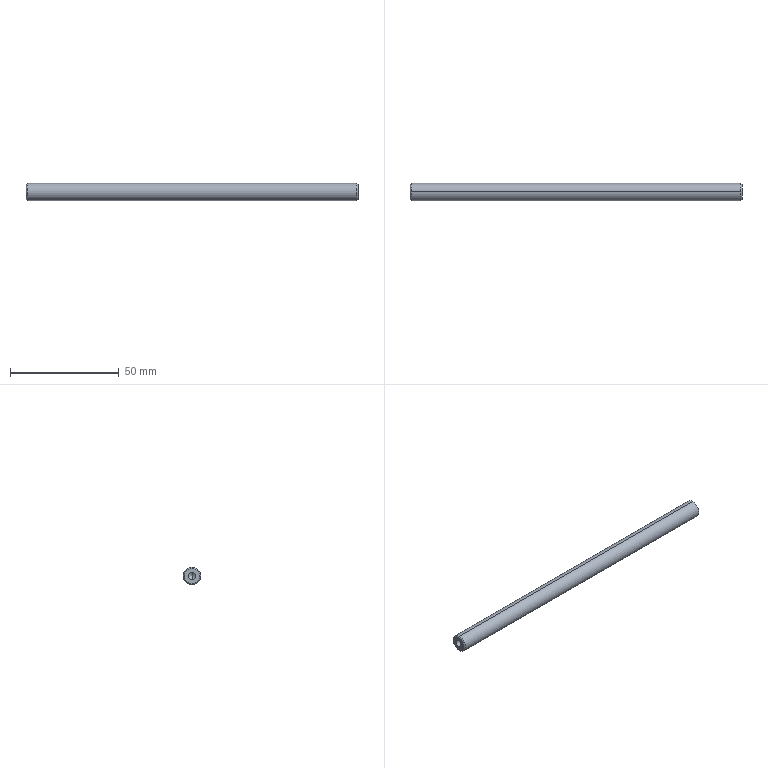Part | STEP file | 03-16 Φ8 column | 1 solid | 16 faces | box 153 x 8 x 8 mm | volume 7438 mm3 | cone 8 | cylinder 6 | plane 2 | commonest cylinder face diameters 3.3 x4 8 x2